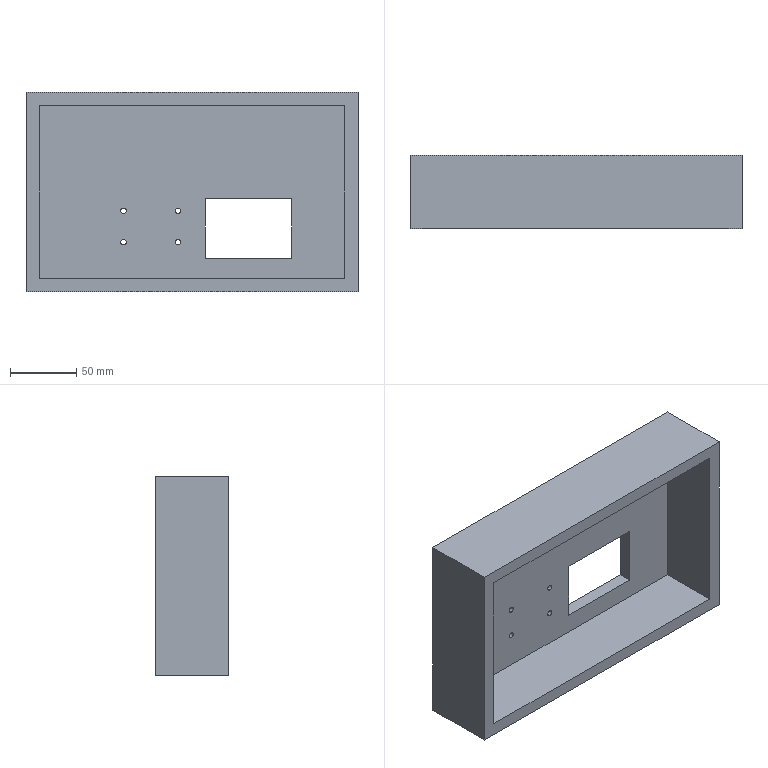Part | SolidWorks | features ICE 2, Cut 1, Extrusion 1 | 1 solid | 23 faces | box 250 x 55 x 150 mm | volume 687196 mm3 | plane 15 | cylinder 8 | commonest cylinder face diameters 4.2 x8
STEP:
#1=CARTESIAN_POINT('',(-42.988,58.447,39.302));
#2=VERTEX_POINT('',#1);
#3=CARTESIAN_POINT('',(-42.988,58.447,35.102));
#4=VERTEX_POINT('',#3);
#5=CARTESIAN_POINT('',(-42.988,58.447,37.202));
#6=DIRECTION('',(0.,-1.,0.));
#7=DIRECTION('',(0.,0.,1.));
#8=AXIS2_PLACEMENT_3D('',#5,#6,#7);
#9=CIRCLE('',#8,2.1);
#10=EDGE_CURVE('',#2,#4,#9,.T.);
#11=ORIENTED_EDGE('',*,*,#10,.T.);
#12=CARTESIAN_POINT('',(-42.988,68.447,35.102));
#13=VERTEX_POINT('',#12);
#14=CARTESIAN_POINT('',(-42.988,52.508,35.102));
#15=DIRECTION('',(0.,1.,0.));
#16=VECTOR('',#15,1000.);
#17=LINE('',#14,#16);
#18=EDGE_CURVE('',#4,#13,#17,.T.);
#19=ORIENTED_EDGE('',*,*,#18,.T.);
#20=CARTESIAN_POINT('',(-42.988,68.447,39.302));
#21=VERTEX_POINT('',#20);
#22=CARTESIAN_POINT('',(-42.988,68.447,37.202));
#23=DIRECTION('',(0.,-1.,0.));
#24=DIRECTION('',(0.,0.,-1.));
#25=AXIS2_PLACEMENT_3D('',#22,#23,#24);
#26=CIRCLE('',#25,2.1);
#27=EDGE_CURVE('',#21,#13,#26,.T.);
#28=ORIENTED_EDGE('',*,*,#27,.F.);
#29=CARTESIAN_POINT('',(-42.988,52.508,39.302));
#30=DIRECTION('',(0.,1.,0.));
#31=VECTOR('',#30,1000.);
#32=LINE('',#29,#31);
#33=EDGE_CURVE('',#2,#21,#32,.T.);
#34=ORIENTED_EDGE('',*,*,#33,.F.);
#35=EDGE_LOOP('',(#11,#19,#28,#34));
#36=FACE_OUTER_BOUND('',#35,.T.);
#37=CARTESIAN_POINT('',(-42.988,52.508,37.202));
#38=DIRECTION('',(0.,1.,0.));
#39=DIRECTION('',(0.,0.,1.));
#40=AXIS2_PLACEMENT_3D('',#37,#38,#39);
#41=CYLINDRICAL_SURFACE('',#40,2.1);
#42=ADVANCED_FACE('',(#36),#41,.F.);
#43=CARTESIAN_POINT('',(-42.988,58.447,62.952));
#44=VERTEX_POINT('',#43);
#45=CARTESIAN_POINT('',(-42.988,58.447,58.752));
#46=VERTEX_POINT('',#45);
#47=CARTESIAN_POINT('',(-42.988,58.447,60.852));
#48=DIRECTION('',(0.,-1.,0.));
#49=DIRECTION('',(0.,0.,1.));
#50=AXIS2_PLACEMENT_3D('',#47,#48,#49);
#51=CIRCLE('',#50,2.1);
#52=EDGE_CURVE('',#44,#46,#51,.T.);
#53=ORIENTED_EDGE('',*,*,#52,.T.);
#54=CARTESIAN_POINT('',(-42.988,68.447,58.752));
#55=VERTEX_POINT('',#54);
#56=CARTESIAN_POINT('',(-42.988,52.508,58.752));
#57=DIRECTION('',(0.,1.,0.));
#58=VECTOR('',#57,1000.);
#59=LINE('',#56,#58);
#60=EDGE_CURVE('',#46,#55,#59,.T.);
#61=ORIENTED_EDGE('',*,*,#60,.T.);
#62=CARTESIAN_POINT('',(-42.988,68.447,62.952));
#63=VERTEX_POINT('',#62);
#64=CARTESIAN_POINT('',(-42.988,68.447,60.852));
#65=DIRECTION('',(0.,-1.,0.));
#66=DIRECTION('',(0.,0.,-1.));
#67=AXIS2_PLACEMENT_3D('',#64,#65,#66);
#68=CIRCLE('',#67,2.1);
#69=EDGE_CURVE('',#63,#55,#68,.T.);
#70=ORIENTED_EDGE('',*,*,#69,.F.);
#71=CARTESIAN_POINT('',(-42.988,52.508,62.952));
#72=DIRECTION('',(0.,1.,0.));
#73=VECTOR('',#72,1000.);
#74=LINE('',#71,#73);
#75=EDGE_CURVE('',#44,#63,#74,.T.);
#76=ORIENTED_EDGE('',*,*,#75,.F.);
#77=EDGE_LOOP('',(#53,#61,#70,#76));
#78=FACE_OUTER_BOUND('',#77,.T.);
#79=CARTESIAN_POINT('',(-42.988,52.508,60.852));
#80=DIRECTION('',(0.,1.,0.));
#81=DIRECTION('',(0.,0.,1.));
#82=AXIS2_PLACEMENT_3D('',#79,#80,#81);
#83=CYLINDRICAL_SURFACE('',#82,2.1);
#84=ADVANCED_FACE('',(#78),#83,.F.);
#85=CARTESIAN_POINT('',(-83.988,58.447,62.952));
#86=VERTEX_POINT('',#85);
#87=CARTESIAN_POINT('',(-83.988,58.447,58.752));
#88=VERTEX_POINT('',#87);
#89=CARTESIAN_POINT('',(-83.988,58.447,60.852));
#90=DIRECTION('',(0.,-1.,0.));
#91=DIRECTION('',(0.,0.,1.));
#92=AXIS2_PLACEMENT_3D('',#89,#90,#91);
#93=CIRCLE('',#92,2.1);
#94=EDGE_CURVE('',#86,#88,#93,.T.);
#95=ORIENTED_EDGE('',*,*,#94,.T.);
#96=CARTESIAN_POINT('',(-83.988,68.447,58.752));
#97=VERTEX_POINT('',#96);
#98=CARTESIAN_POINT('',(-83.988,52.508,58.752));
#99=DIRECTION('',(0.,1.,0.));
#100=VECTOR('',#99,1000.);
#101=LINE('',#98,#100);
#102=EDGE_CURVE('',#88,#97,#101,.T.);
#103=ORIENTED_EDGE('',*,*,#102,.T.);
#104=CARTESIAN_POINT('',(-83.988,68.447,62.952));
#105=VERTEX_POINT('',#104);
#106=CARTESIAN_POINT('',(-83.988,68.447,60.852));
#107=DIRECTION('',(0.,-1.,0.));
#108=DIRECTION('',(0.,0.,-1.));
#109=AXIS2_PLACEMENT_3D('',#106,#107,#108);
#110=CIRCLE('',#109,2.1);
#111=EDGE_CURVE('',#105,#97,#110,.T.);
#112=ORIENTED_EDGE('',*,*,#111,.F.);
#113=CARTESIAN_POINT('',(-83.988,52.508,62.952));
#114=DIRECTION('',(0.,1.,0.));
#115=VECTOR('',#114,1000.);
#116=LINE('',#113,#115);
#117=EDGE_CURVE('',#86,#105,#116,.T.);
#118=ORIENTED_EDGE('',*,*,#117,.F.);
#119=EDGE_LOOP('',(#95,#103,#112,#118));
#120=FACE_OUTER_BOUND('',#119,.T.);
#121=CARTESIAN_POINT('',(-83.988,52.508,60.852));
#122=DIRECTION('',(0.,1.,0.));
#123=DIRECTION('',(0.,0.,1.));
#124=AXIS2_PLACEMENT_3D('',#121,#122,#123);
#125=CYLINDRICAL_SURFACE('',#124,2.1);
#126=ADVANCED_FACE('',(#120),#125,.F.);
#127=CARTESIAN_POINT('',(-83.988,58.447,39.302));
#128=VERTEX_POINT('',#127);
#129=CARTESIAN_POINT('',(-83.988,58.447,35.102));
#130=VERTEX_POINT('',#129);
#131=CARTESIAN_POINT('',(-83.988,58.447,37.202));
#132=DIRECTION('',(0.,-1.,0.));
#133=DIRECTION('',(0.,0.,1.));
#134=AXIS2_PLACEMENT_3D('',#131,#132,#133);
#135=CIRCLE('',#134,2.1);
#136=EDGE_CURVE('',#128,#130,#135,.T.);
#137=ORIENTED_EDGE('',*,*,#136,.T.);
#138=CARTESIAN_POINT('',(-83.988,68.447,35.102));
#139=VERTEX_POINT('',#138);
#140=CARTESIAN_POINT('',(-83.988,52.508,35.102));
#141=DIRECTION('',(0.,1.,0.));
#142=VECTOR('',#141,1000.);
#143=LINE('',#140,#142);
#144=EDGE_CURVE('',#130,#139,#143,.T.);
#145=ORIENTED_EDGE('',*,*,#144,.T.);
#146=CARTESIAN_POINT('',(-83.988,68.447,39.302));
#147=VERTEX_POINT('',#146);
#148=CARTESIAN_POINT('',(-83.988,68.447,37.202));
#149=DIRECTION('',(0.,-1.,0.));
#150=DIRECTION('',(0.,0.,-1.));
#151=AXIS2_PLACEMENT_3D('',#148,#149,#150);
#152=CIRCLE('',#151,2.1);
#153=EDGE_CURVE('',#147,#139,#152,.T.);
#154=ORIENTED_EDGE('',*,*,#153,.F.);
#155=CARTESIAN_POINT('',(-83.988,52.508,39.302));
#156=DIRECTION('',(0.,1.,0.));
#157=VECTOR('',#156,1000.);
#158=LINE('',#155,#157);
#159=EDGE_CURVE('',#128,#147,#158,.T.);
#160=ORIENTED_EDGE('',*,*,#159,.F.);
#161=EDGE_LOOP('',(#137,#145,#154,#160));
#162=FACE_OUTER_BOUND('',#161,.T.);
#163=CARTESIAN_POINT('',(-83.988,52.508,37.202));
#164=DIRECTION('',(0.,1.,0.));
#165=DIRECTION('',(0.,0.,1.));
#166=AXIS2_PLACEMENT_3D('',#163,#164,#165);
#167=CYLINDRICAL_SURFACE('',#166,2.1);
#168=ADVANCED_FACE('',(#162),#167,.F.);
#169=CARTESIAN_POINT('',(-157.482,68.447,0.));
#170=VERTEX_POINT('',#169);
#171=CARTESIAN_POINT('',(-157.482,13.447,0.));
#172=VERTEX_POINT('',#171);
#173=CARTESIAN_POINT('',(-157.482,68.447,0.));
#174=DIRECTION('',(0.,-1.,0.));
#175=VECTOR('',#174,1000.);
#176=LINE('',#173,#175);
#177=EDGE_CURVE('',#170,#172,#176,.T.);
#178=ORIENTED_EDGE('',*,*,#177,.T.);
#179=CARTESIAN_POINT('',(-157.482,13.447,150.));
#180=VERTEX_POINT('',#179);
#181=CARTESIAN_POINT('',(-157.482,13.447,150.));
#182=DIRECTION('',(0.,0.,-1.));
#183=VECTOR('',#182,1000.);
#184=LINE('',#181,#183);
#185=EDGE_CURVE('',#180,#172,#184,.T.);
#186=ORIENTED_EDGE('',*,*,#185,.F.);
#187=CARTESIAN_POINT('',(-157.482,68.447,150.));
#188=VERTEX_POINT('',#187);
#189=CARTESIAN_POINT('',(-157.482,68.447,150.));
#190=DIRECTION('',(0.,-1.,0.));
#191=VECTOR('',#190,1000.);
#192=LINE('',#189,#191);
#193=EDGE_CURVE('',#188,#180,#192,.T.);
#194=ORIENTED_EDGE('',*,*,#193,.F.);
#195=CARTESIAN_POINT('',(-157.482,68.447,150.));
#196=DIRECTION('',(0.,0.,-1.));
#197=VECTOR('',#196,1000.);
#198=LINE('',#195,#197);
#199=EDGE_CURVE('',#188,#170,#198,.T.);
#200=ORIENTED_EDGE('',*,*,#199,.T.);
#201=EDGE_LOOP('',(#178,#186,#194,#200));
#202=FACE_OUTER_BOUND('',#201,.T.);
#203=CARTESIAN_POINT('',(-157.482,68.447,150.));
#204=DIRECTION('',(1.,0.,0.));
#205=DIRECTION('',(0.,0.,-1.));
#206=AXIS2_PLACEMENT_3D('',#203,#204,#205);
#207=PLANE('',#206);
#208=ADVANCED_FACE('',(#202),#207,.F.);
#209=CARTESIAN_POINT('',(-147.482,13.447,10.));
#210=VERTEX_POINT('',#209);
#211=CARTESIAN_POINT('',(82.518,13.447,10.));
#212=VERTEX_POINT('',#211);
#213=CARTESIAN_POINT('',(82.518,13.447,10.));
#214=DIRECTION('',(1.,0.,0.));
#215=VECTOR('',#214,1000.);
#216=LINE('',#213,#215);
#217=EDGE_CURVE('',#210,#212,#216,.T.);
#218=ORIENTED_EDGE('',*,*,#217,.F.);
#219=CARTESIAN_POINT('',(-147.482,13.447,140.));
#220=VERTEX_POINT('',#219);
#221=CARTESIAN_POINT('',(-147.482,13.447,140.));
#222=DIRECTION('',(0.,0.,-1.));
#223=VECTOR('',#222,1000.);
#224=LINE('',#221,#223);
#225=EDGE_CURVE('',#220,#210,#224,.T.);
#226=ORIENTED_EDGE('',*,*,#225,.F.);
#227=CARTESIAN_POINT('',(82.518,13.447,140.));
#228=VERTEX_POINT('',#227);
#229=CARTESIAN_POINT('',(-147.482,13.447,140.));
#230=DIRECTION('',(-1.,0.,0.));
#231=VECTOR('',#230,1000.);
#232=LINE('',#229,#231);
#233=EDGE_CURVE('',#228,#220,#232,.T.);
#234=ORIENTED_EDGE('',*,*,#233,.F.);
#235=CARTESIAN_POINT('',(82.518,13.447,140.));
#236=DIRECTION('',(0.,0.,1.));
#237=VECTOR('',#236,1000.);
#238=LINE('',#235,#237);
#239=EDGE_CURVE('',#212,#228,#238,.T.);
#240=ORIENTED_EDGE('',*,*,#239,.F.);
#241=EDGE_LOOP('',(#218,#226,#234,#240));
#242=FACE_BOUND('',#241,.T.);
#243=CARTESIAN_POINT('',(92.518,13.447,0.));
#244=VERTEX_POINT('',#243);
#245=CARTESIAN_POINT('',(-157.482,13.447,0.));
#246=DIRECTION('',(1.,0.,0.));
#247=VECTOR('',#246,1000.);
#248=LINE('',#245,#247);
#249=EDGE_CURVE('',#172,#244,#248,.T.);
#250=ORIENTED_EDGE('',*,*,#249,.T.);
#251=CARTESIAN_POINT('',(92.518,13.447,150.));
#252=VERTEX_POINT('',#251);
#253=CARTESIAN_POINT('',(92.518,13.447,150.));
#254=DIRECTION('',(0.,0.,-1.));
#255=VECTOR('',#254,1000.);
#256=LINE('',#253,#255);
#257=EDGE_CURVE('',#252,#244,#256,.T.);
#258=ORIENTED_EDGE('',*,*,#257,.F.);
#259=CARTESIAN_POINT('',(-157.482,13.447,150.));
#260=DIRECTION('',(1.,0.,0.));
#261=VECTOR('',#260,1000.);
#262=LINE('',#259,#261);
#263=EDGE_CURVE('',#180,#252,#262,.T.);
#264=ORIENTED_EDGE('',*,*,#263,.F.);
#265=ORIENTED_EDGE('',*,*,#185,.T.);
#266=EDGE_LOOP('',(#250,#258,#264,#265));
#267=FACE_OUTER_BOUND('',#266,.T.);
#268=CARTESIAN_POINT('',(-157.482,13.447,150.));
#269=DIRECTION('',(0.,1.,0.));
#270=DIRECTION('',(0.,0.,1.));
#271=AXIS2_PLACEMENT_3D('',#268,#269,#270);
#272=PLANE('',#271);
#273=ADVANCED_FACE('',(#242,#267),#272,.F.);
#274=CARTESIAN_POINT('',(92.518,68.447,0.));
#275=VERTEX_POINT('',#274);
#276=CARTESIAN_POINT('',(92.518,68.447,0.));
#277=DIRECTION('',(0.,1.,0.));
#278=VECTOR('',#277,1000.);
#279=LINE('',#276,#278);
#280=EDGE_CURVE('',#244,#275,#279,.T.);
#281=ORIENTED_EDGE('',*,*,#280,.T.);
#282=CARTESIAN_POINT('',(92.518,68.447,150.));
#283=VERTEX_POINT('',#282);
#284=CARTESIAN_POINT('',(92.518,68.447,150.));
#285=DIRECTION('',(0.,0.,-1.));
#286=VECTOR('',#285,1000.);
#287=LINE('',#284,#286);
#288=EDGE_CURVE('',#283,#275,#287,.T.);
#289=ORIENTED_EDGE('',*,*,#288,.F.);
#290=CARTESIAN_POINT('',(92.518,68.447,150.));
#291=DIRECTION('',(0.,1.,0.));
#292=VECTOR('',#291,1000.);
#293=LINE('',#290,#292);
#294=EDGE_CURVE('',#252,#283,#293,.T.);
#295=ORIENTED_EDGE('',*,*,#294,.F.);
#296=ORIENTED_EDGE('',*,*,#257,.T.);
#297=EDGE_LOOP('',(#281,#289,#295,#296));
#298=FACE_OUTER_BOUND('',#297,.T.);
#299=CARTESIAN_POINT('',(92.518,68.447,150.));
#300=DIRECTION('',(-1.,0.,0.));
#301=DIRECTION('',(0.,-1.,0.));
#302=AXIS2_PLACEMENT_3D('',#299,#300,#301);
#303=PLANE('',#302);
#304=ADVANCED_FACE('',(#298),#303,.F.);
#305=ORIENTED_EDGE('',*,*,#27,.T.);
#306=CARTESIAN_POINT('',(-42.988,68.447,37.202));
#307=DIRECTION('',(0.,-1.,0.));
#308=DIRECTION('',(0.,0.,-1.));
#309=AXIS2_PLACEMENT_3D('',#306,#307,#308);
#310=CIRCLE('',#309,2.1);
#311=EDGE_CURVE('',#13,#21,#310,.T.);
#312=ORIENTED_EDGE('',*,*,#311,.T.);
#313=EDGE_LOOP('',(#305,#312));
#314=FACE_BOUND('',#313,.T.);
#315=ORIENTED_EDGE('',*,*,#69,.T.);
#316=CARTESIAN_POINT('',(-42.988,68.447,60.852));
#317=DIRECTION('',(0.,-1.,0.));
#318=DIRECTION('',(0.,0.,-1.));
#319=AXIS2_PLACEMENT_3D('',#316,#317,#318);
#320=CIRCLE('',#319,2.1);
#321=EDGE_CURVE('',#55,#63,#320,.T.);
#322=ORIENTED_EDGE('',*,*,#321,.T.);
#323=EDGE_LOOP('',(#315,#322));
#324=FACE_BOUND('',#323,.T.);
#325=ORIENTED_EDGE('',*,*,#111,.T.);
#326=CARTESIAN_POINT('',(-83.988,68.447,60.852));
#327=DIRECTION('',(0.,-1.,0.));
#328=DIRECTION('',(0.,0.,-1.));
#329=AXIS2_PLACEMENT_3D('',#326,#327,#328);
#330=CIRCLE('',#329,2.1);
#331=EDGE_CURVE('',#97,#105,#330,.T.);
#332=ORIENTED_EDGE('',*,*,#331,.T.);
#333=EDGE_LOOP('',(#325,#332));
#334=FACE_BOUND('',#333,.T.);
#335=ORIENTED_EDGE('',*,*,#153,.T.);
#336=CARTESIAN_POINT('',(-83.988,68.447,37.202));
#337=DIRECTION('',(0.,-1.,0.));
#338=DIRECTION('',(0.,0.,-1.));
#339=AXIS2_PLACEMENT_3D('',#336,#337,#338);
#340=CIRCLE('',#339,2.1);
#341=EDGE_CURVE('',#139,#147,#340,.T.);
#342=ORIENTED_EDGE('',*,*,#341,.T.);
#343=EDGE_LOOP('',(#335,#342));
#344=FACE_BOUND('',#343,.T.);
#345=CARTESIAN_POINT('',(42.518,68.447,70.));
#346=VERTEX_POINT('',#345);
#347=CARTESIAN_POINT('',(-22.482,68.447,70.));
#348=VERTEX_POINT('',#347);
#349=CARTESIAN_POINT('',(-22.482,68.447,70.));
#350=DIRECTION('',(-1.,0.,0.));
#351=VECTOR('',#350,1000.);
#352=LINE('',#349,#351);
#353=EDGE_CURVE('',#346,#348,#352,.T.);
#354=ORIENTED_EDGE('',*,*,#353,.T.);
#355=CARTESIAN_POINT('',(-22.482,68.447,25.));
#356=VERTEX_POINT('',#355);
#357=CARTESIAN_POINT('',(-22.482,68.447,70.));
#358=DIRECTION('',(0.,0.,-1.));
#359=VECTOR('',#358,1000.);
#360=LINE('',#357,#359);
#361=EDGE_CURVE('',#348,#356,#360,.T.);
#362=ORIENTED_EDGE('',*,*,#361,.T.);
#363=CARTESIAN_POINT('',(42.518,68.447,25.));
#364=VERTEX_POINT('',#363);
#365=CARTESIAN_POINT('',(-22.482,68.447,25.));
#366=DIRECTION('',(1.,0.,0.));
#367=VECTOR('',#366,1000.);
#368=LINE('',#365,#367);
#369=EDGE_CURVE('',#356,#364,#368,.T.);
#370=ORIENTED_EDGE('',*,*,#369,.T.);
#371=CARTESIAN_POINT('',(42.518,68.447,70.));
#372=DIRECTION('',(0.,0.,1.));
#373=VECTOR('',#372,1000.);
#374=LINE('',#371,#373);
#375=EDGE_CURVE('',#364,#346,#374,.T.);
#376=ORIENTED_EDGE('',*,*,#375,.T.);
#377=EDGE_LOOP('',(#354,#362,#370,#376));
#378=FACE_BOUND('',#377,.T.);
#379=CARTESIAN_POINT('',(-157.482,68.447,0.));
#380=DIRECTION('',(-1.,0.,0.));
#381=VECTOR('',#380,1000.);
#382=LINE('',#379,#381);
#383=EDGE_CURVE('',#275,#170,#382,.T.);
#384=ORIENTED_EDGE('',*,*,#383,.T.);
#385=ORIENTED_EDGE('',*,*,#199,.F.);
#386=CARTESIAN_POINT('',(-157.482,68.447,150.));
#387=DIRECTION('',(-1.,0.,0.));
#388=VECTOR('',#387,1000.);
#389=LINE('',#386,#388);
#390=EDGE_CURVE('',#283,#188,#389,.T.);
#391=ORIENTED_EDGE('',*,*,#390,.F.);
#392=ORIENTED_EDGE('',*,*,#288,.T.);
#393=EDGE_LOOP('',(#384,#385,#391,#392));
#394=FACE_OUTER_BOUND('',#393,.T.);
#395=CARTESIAN_POINT('',(-157.482,68.447,150.));
#396=DIRECTION('',(0.,-1.,0.));
#397=DIRECTION('',(0.,0.,-1.));
#398=AXIS2_PLACEMENT_3D('',#395,#396,#397);
#399=PLANE('',#398);
#400=ADVANCED_FACE('',(#314,#324,#334,#344,#378,#394),#399,.F.);
#401=ORIENTED_EDGE('',*,*,#193,.T.);
#402=ORIENTED_EDGE('',*,*,#263,.T.);
#403=ORIENTED_EDGE('',*,*,#294,.T.);
#404=ORIENTED_EDGE('',*,*,#390,.T.);
#405=EDGE_LOOP('',(#401,#402,#403,#404));
#406=FACE_OUTER_BOUND('',#405,.T.);
#407=CARTESIAN_POINT('',(0.,0.,150.));
#408=DIRECTION('',(0.,0.,1.));
#409=DIRECTION('',(1.,0.,0.));
#410=AXIS2_PLACEMENT_3D('',#407,#408,#409);
#411=PLANE('',#410);
#412=ADVANCED_FACE('',(#406),#411,.T.);
#413=ORIENTED_EDGE('',*,*,#177,.F.);
#414=ORIENTED_EDGE('',*,*,#383,.F.);
#415=ORIENTED_EDGE('',*,*,#280,.F.);
#416=ORIENTED_EDGE('',*,*,#249,.F.);
#417=EDGE_LOOP('',(#413,#414,#415,#416));
#418=FACE_OUTER_BOUND('',#417,.T.);
#419=CARTESIAN_POINT('',(0.,0.,0.));
#420=DIRECTION('',(0.,0.,1.));
#421=DIRECTION('',(1.,0.,0.));
#422=AXIS2_PLACEMENT_3D('',#419,#420,#421);
#423=PLANE('',#422);
#424=ADVANCED_FACE('',(#418),#423,.F.);
#425=ORIENTED_EDGE('',*,*,#225,.T.);
#426=CARTESIAN_POINT('',(-147.482,58.447,10.));
#427=VERTEX_POINT('',#426);
#428=CARTESIAN_POINT('',(-147.482,58.447,10.));
#429=DIRECTION('',(0.,-1.,0.));
#430=VECTOR('',#429,1000.);
#431=LINE('',#428,#430);
#432=EDGE_CURVE('',#427,#210,#431,.T.);
#433=ORIENTED_EDGE('',*,*,#432,.F.);
#434=CARTESIAN_POINT('',(-147.482,58.447,140.));
#435=VERTEX_POINT('',#434);
#436=CARTESIAN_POINT('',(-147.482,58.447,140.));
#437=DIRECTION('',(0.,0.,-1.));
#438=VECTOR('',#437,1000.);
#439=LINE('',#436,#438);
#440=EDGE_CURVE('',#435,#427,#439,.T.);
#441=ORIENTED_EDGE('',*,*,#440,.F.);
#442=CARTESIAN_POINT('',(-147.482,58.447,140.));
#443=DIRECTION('',(0.,-1.,0.));
#444=VECTOR('',#443,1000.);
#445=LINE('',#442,#444);
#446=EDGE_CURVE('',#435,#220,#445,.T.);
#447=ORIENTED_EDGE('',*,*,#446,.T.);
#448=EDGE_LOOP('',(#425,#433,#441,#447));
#449=FACE_OUTER_BOUND('',#448,.T.);
#450=CARTESIAN_POINT('',(-147.482,58.447,140.));
#451=DIRECTION('',(-1.,0.,0.));
#452=DIRECTION('',(0.,0.,1.));
#453=AXIS2_PLACEMENT_3D('',#450,#451,#452);
#454=PLANE('',#453);
#455=ADVANCED_FACE('',(#449),#454,.F.);
#456=ORIENTED_EDGE('',*,*,#233,.T.);
#457=ORIENTED_EDGE('',*,*,#446,.F.);
#458=CARTESIAN_POINT('',(82.518,58.447,140.));
#459=VERTEX_POINT('',#458);
#460=CARTESIAN_POINT('',(-147.482,58.447,140.));
#461=DIRECTION('',(-1.,0.,0.));
#462=VECTOR('',#461,1000.);
#463=LINE('',#460,#462);
#464=EDGE_CURVE('',#459,#435,#463,.T.);
#465=ORIENTED_EDGE('',*,*,#464,.F.);
#466=CARTESIAN_POINT('',(82.518,58.447,140.));
#467=DIRECTION('',(0.,-1.,0.));
#468=VECTOR('',#467,1000.);
#469=LINE('',#466,#468);
#470=EDGE_CURVE('',#459,#228,#469,.T.);
#471=ORIENTED_EDGE('',*,*,#470,.T.);
#472=EDGE_LOOP('',(#456,#457,#465,#471));
#473=FACE_OUTER_BOUND('',#472,.T.);
#474=CARTESIAN_POINT('',(-147.482,58.447,140.));
#475=DIRECTION('',(0.,0.,1.));
#476=DIRECTION('',(1.,0.,0.));
#477=AXIS2_PLACEMENT_3D('',#474,#475,#476);
#478=PLANE('',#477);
#479=ADVANCED_FACE('',(#473),#478,.F.);
#480=ORIENTED_EDGE('',*,*,#239,.T.);
#481=ORIENTED_EDGE('',*,*,#470,.F.);
#482=CARTESIAN_POINT('',(82.518,58.447,10.));
#483=VERTEX_POINT('',#482);
#484=CARTESIAN_POINT('',(82.518,58.447,140.));
#485=DIRECTION('',(0.,0.,1.));
#486=VECTOR('',#485,1000.);
#487=LINE('',#484,#486);
#488=EDGE_CURVE('',#483,#459,#487,.T.);
#489=ORIENTED_EDGE('',*,*,#488,.F.);
#490=CARTESIAN_POINT('',(82.518,58.447,10.));
#491=DIRECTION('',(0.,-1.,0.));
#492=VECTOR('',#491,1000.);
#493=LINE('',#490,#492);
#494=EDGE_CURVE('',#483,#212,#493,.T.);
#495=ORIENTED_EDGE('',*,*,#494,.T.);
#496=EDGE_LOOP('',(#480,#481,#489,#495));
#497=FACE_OUTER_BOUND('',#496,.T.);
#498=CARTESIAN_POINT('',(82.518,58.447,140.));
#499=DIRECTION('',(1.,0.,0.));
#500=DIRECTION('',(0.,0.,-1.));
#501=AXIS2_PLACEMENT_3D('',#498,#499,#500);
#502=PLANE('',#501);
#503=ADVANCED_FACE('',(#497),#502,.F.);
#504=ORIENTED_EDGE('',*,*,#217,.T.);
#505=ORIENTED_EDGE('',*,*,#494,.F.);
#506=CARTESIAN_POINT('',(82.518,58.447,10.));
#507=DIRECTION('',(1.,0.,0.));
#508=VECTOR('',#507,1000.);
#509=LINE('',#506,#508);
#510=EDGE_CURVE('',#427,#483,#509,.T.);
#511=ORIENTED_EDGE('',*,*,#510,.F.);
#512=ORIENTED_EDGE('',*,*,#432,.T.);
#513=EDGE_LOOP('',(#504,#505,#511,#512));
#514=FACE_OUTER_BOUND('',#513,.T.);
#515=CARTESIAN_POINT('',(82.518,58.447,10.));
#516=DIRECTION('',(0.,0.,-1.));
#517=DIRECTION('',(-1.,0.,0.));
#518=AXIS2_PLACEMENT_3D('',#515,#516,#517);
#519=PLANE('',#518);
#520=ADVANCED_FACE('',(#514),#519,.F.);
#521=ORIENTED_EDGE('',*,*,#10,.F.);
#522=CARTESIAN_POINT('',(-42.988,58.447,37.202));
#523=DIRECTION('',(0.,-1.,0.));
#524=DIRECTION('',(0.,0.,1.));
#525=AXIS2_PLACEMENT_3D('',#522,#523,#524);
#526=CIRCLE('',#525,2.1);
#527=EDGE_CURVE('',#4,#2,#526,.T.);
#528=ORIENTED_EDGE('',*,*,#527,.F.);
#529=EDGE_LOOP('',(#521,#528));
#530=FACE_BOUND('',#529,.T.);
#531=ORIENTED_EDGE('',*,*,#52,.F.);
#532=CARTESIAN_POINT('',(-42.988,58.447,60.852));
#533=DIRECTION('',(0.,-1.,0.));
#534=DIRECTION('',(0.,0.,1.));
#535=AXIS2_PLACEMENT_3D('',#532,#533,#534);
#536=CIRCLE('',#535,2.1);
#537=EDGE_CURVE('',#46,#44,#536,.T.);
#538=ORIENTED_EDGE('',*,*,#537,.F.);
#539=EDGE_LOOP('',(#531,#538));
#540=FACE_BOUND('',#539,.T.);
#541=ORIENTED_EDGE('',*,*,#94,.F.);
#542=CARTESIAN_POINT('',(-83.988,58.447,60.852));
#543=DIRECTION('',(0.,-1.,0.));
#544=DIRECTION('',(0.,0.,1.));
#545=AXIS2_PLACEMENT_3D('',#542,#543,#544);
#546=CIRCLE('',#545,2.1);
#547=EDGE_CURVE('',#88,#86,#546,.T.);
#548=ORIENTED_EDGE('',*,*,#547,.F.);
#549=EDGE_LOOP('',(#541,#548));
#550=FACE_BOUND('',#549,.T.);
#551=ORIENTED_EDGE('',*,*,#136,.F.);
#552=CARTESIAN_POINT('',(-83.988,58.447,37.202));
#553=DIRECTION('',(0.,-1.,0.));
#554=DIRECTION('',(0.,0.,1.));
#555=AXIS2_PLACEMENT_3D('',#552,#553,#554);
#556=CIRCLE('',#555,2.1);
#557=EDGE_CURVE('',#130,#128,#556,.T.);
#558=ORIENTED_EDGE('',*,*,#557,.F.);
#559=EDGE_LOOP('',(#551,#558));
#560=FACE_BOUND('',#559,.T.);
#561=CARTESIAN_POINT('',(-22.482,58.447,25.));
#562=VERTEX_POINT('',#561);
#563=CARTESIAN_POINT('',(42.518,58.447,25.));
#564=VERTEX_POINT('',#563);
#565=CARTESIAN_POINT('',(-22.482,58.447,25.));
#566=DIRECTION('',(1.,0.,0.));
#567=VECTOR('',#566,1000.);
#568=LINE('',#565,#567);
#569=EDGE_CURVE('',#562,#564,#568,.T.);
#570=ORIENTED_EDGE('',*,*,#569,.F.);
#571=CARTESIAN_POINT('',(-22.482,58.447,70.));
#572=VERTEX_POINT('',#571);
#573=CARTESIAN_POINT('',(-22.482,58.447,70.));
#574=DIRECTION('',(0.,0.,-1.));
#575=VECTOR('',#574,1000.);
#576=LINE('',#573,#575);
#577=EDGE_CURVE('',#572,#562,#576,.T.);
#578=ORIENTED_EDGE('',*,*,#577,.F.);
#579=CARTESIAN_POINT('',(42.518,58.447,70.));
#580=VERTEX_POINT('',#579);
#581=CARTESIAN_POINT('',(-22.482,58.447,70.));
#582=DIRECTION('',(-1.,0.,0.));
#583=VECTOR('',#582,1000.);
#584=LINE('',#581,#583);
#585=EDGE_CURVE('',#580,#572,#584,.T.);
#586=ORIENTED_EDGE('',*,*,#585,.F.);
#587=CARTESIAN_POINT('',(42.518,58.447,70.));
#588=DIRECTION('',(0.,0.,1.));
#589=VECTOR('',#588,1000.);
#590=LINE('',#587,#589);
#591=EDGE_CURVE('',#564,#580,#590,.T.);
#592=ORIENTED_EDGE('',*,*,#591,.F.);
#593=EDGE_LOOP('',(#570,#578,#586,#592));
#594=FACE_BOUND('',#593,.T.);
#595=ORIENTED_EDGE('',*,*,#440,.T.);
#596=ORIENTED_EDGE('',*,*,#510,.T.);
#597=ORIENTED_EDGE('',*,*,#488,.T.);
#598=ORIENTED_EDGE('',*,*,#464,.T.);
#599=EDGE_LOOP('',(#595,#596,#597,#598));
#600=FACE_OUTER_BOUND('',#599,.T.);
#601=CARTESIAN_POINT('',(0.,58.447,0.));
#602=DIRECTION('',(0.,1.,0.));
#603=DIRECTION('',(0.,0.,1.));
#604=AXIS2_PLACEMENT_3D('',#601,#602,#603);
#605=PLANE('',#604);
#606=ADVANCED_FACE('',(#530,#540,#550,#560,#594,#600),#605,.F.);
#607=ORIENTED_EDGE('',*,*,#577,.T.);
#608=CARTESIAN_POINT('',(-22.482,68.447,25.));
#609=DIRECTION('',(0.,-1.,0.));
#610=VECTOR('',#609,1000.);
#611=LINE('',#608,#610);
#612=EDGE_CURVE('',#356,#562,#611,.T.);
#613=ORIENTED_EDGE('',*,*,#612,.F.);
#614=ORIENTED_EDGE('',*,*,#361,.F.);
#615=CARTESIAN_POINT('',(-22.482,68.447,70.));
#616=DIRECTION('',(0.,-1.,0.));
#617=VECTOR('',#616,1000.);
#618=LINE('',#615,#617);
#619=EDGE_CURVE('',#348,#572,#618,.T.);
#620=ORIENTED_EDGE('',*,*,#619,.T.);
#621=EDGE_LOOP('',(#607,#613,#614,#620));
#622=FACE_OUTER_BOUND('',#621,.T.);
#623=CARTESIAN_POINT('',(-22.482,68.447,70.));
#624=DIRECTION('',(-1.,0.,0.));
#625=DIRECTION('',(0.,0.,1.));
#626=AXIS2_PLACEMENT_3D('',#623,#624,#625);
#627=PLANE('',#626);
#628=ADVANCED_FACE('',(#622),#627,.F.);
#629=ORIENTED_EDGE('',*,*,#585,.T.);
#630=ORIENTED_EDGE('',*,*,#619,.F.);
#631=ORIENTED_EDGE('',*,*,#353,.F.);
#632=CARTESIAN_POINT('',(42.518,68.447,70.));
#633=DIRECTION('',(0.,-1.,0.));
#634=VECTOR('',#633,1000.);
#635=LINE('',#632,#634);
#636=EDGE_CURVE('',#346,#580,#635,.T.);
#637=ORIENTED_EDGE('',*,*,#636,.T.);
#638=EDGE_LOOP('',(#629,#630,#631,#637));
#639=FACE_OUTER_BOUND('',#638,.T.);
#640=CARTESIAN_POINT('',(-22.482,68.447,70.));
#641=DIRECTION('',(0.,0.,1.));
#642=DIRECTION('',(1.,0.,0.));
#643=AXIS2_PLACEMENT_3D('',#640,#641,#642);
#644=PLANE('',#643);
#645=ADVANCED_FACE('',(#639),#644,.F.);
#646=ORIENTED_EDGE('',*,*,#591,.T.);
#647=ORIENTED_EDGE('',*,*,#636,.F.);
#648=ORIENTED_EDGE('',*,*,#375,.F.);
#649=CARTESIAN_POINT('',(42.518,68.447,25.));
#650=DIRECTION('',(0.,-1.,0.));
#651=VECTOR('',#650,1000.);
#652=LINE('',#649,#651);
#653=EDGE_CURVE('',#364,#564,#652,.T.);
#654=ORIENTED_EDGE('',*,*,#653,.T.);
#655=EDGE_LOOP('',(#646,#647,#648,#654));
#656=FACE_OUTER_BOUND('',#655,.T.);
#657=CARTESIAN_POINT('',(42.518,68.447,70.));
#658=DIRECTION('',(1.,0.,0.));
#659=DIRECTION('',(0.,0.,-1.));
#660=AXIS2_PLACEMENT_3D('',#657,#658,#659);
#661=PLANE('',#660);
#662=ADVANCED_FACE('',(#656),#661,.F.);
#663=ORIENTED_EDGE('',*,*,#569,.T.);
#664=ORIENTED_EDGE('',*,*,#653,.F.);
#665=ORIENTED_EDGE('',*,*,#369,.F.);
#666=ORIENTED_EDGE('',*,*,#612,.T.);
#667=EDGE_LOOP('',(#663,#664,#665,#666));
#668=FACE_OUTER_BOUND('',#667,.T.);
#669=CARTESIAN_POINT('',(-22.482,68.447,25.));
#670=DIRECTION('',(0.,0.,-1.));
#671=DIRECTION('',(-1.,0.,0.));
#672=AXIS2_PLACEMENT_3D('',#669,#670,#671);
#673=PLANE('',#672);
#674=ADVANCED_FACE('',(#668),#673,.F.);
#675=ORIENTED_EDGE('',*,*,#144,.F.);
#676=ORIENTED_EDGE('',*,*,#557,.T.);
#677=ORIENTED_EDGE('',*,*,#159,.T.);
#678=ORIENTED_EDGE('',*,*,#341,.F.);
#679=EDGE_LOOP('',(#675,#676,#677,#678));
#680=FACE_OUTER_BOUND('',#679,.T.);
#681=CARTESIAN_POINT('',(-83.988,52.508,37.202));
#682=DIRECTION('',(0.,1.,0.));
#683=DIRECTION('',(0.,0.,1.));
#684=AXIS2_PLACEMENT_3D('',#681,#682,#683);
#685=CYLINDRICAL_SURFACE('',#684,2.1);
#686=ADVANCED_FACE('',(#680),#685,.F.);
#687=ORIENTED_EDGE('',*,*,#102,.F.);
#688=ORIENTED_EDGE('',*,*,#547,.T.);
#689=ORIENTED_EDGE('',*,*,#117,.T.);
#690=ORIENTED_EDGE('',*,*,#331,.F.);
#691=EDGE_LOOP('',(#687,#688,#689,#690));
#692=FACE_OUTER_BOUND('',#691,.T.);
#693=CARTESIAN_POINT('',(-83.988,52.508,60.852));
#694=DIRECTION('',(0.,1.,0.));
#695=DIRECTION('',(0.,0.,1.));
#696=AXIS2_PLACEMENT_3D('',#693,#694,#695);
#697=CYLINDRICAL_SURFACE('',#696,2.1);
#698=ADVANCED_FACE('',(#692),#697,.F.);
#699=ORIENTED_EDGE('',*,*,#60,.F.);
#700=ORIENTED_EDGE('',*,*,#537,.T.);
#701=ORIENTED_EDGE('',*,*,#75,.T.);
#702=ORIENTED_EDGE('',*,*,#321,.F.);
#703=EDGE_LOOP('',(#699,#700,#701,#702));
#704=FACE_OUTER_BOUND('',#703,.T.);
#705=CARTESIAN_POINT('',(-42.988,52.508,60.852));
#706=DIRECTION('',(0.,1.,0.));
#707=DIRECTION('',(0.,0.,1.));
#708=AXIS2_PLACEMENT_3D('',#705,#706,#707);
#709=CYLINDRICAL_SURFACE('',#708,2.1);
#710=ADVANCED_FACE('',(#704),#709,.F.);
#711=ORIENTED_EDGE('',*,*,#18,.F.);
#712=ORIENTED_EDGE('',*,*,#527,.T.);
#713=ORIENTED_EDGE('',*,*,#33,.T.);
#714=ORIENTED_EDGE('',*,*,#311,.F.);
#715=EDGE_LOOP('',(#711,#712,#713,#714));
#716=FACE_OUTER_BOUND('',#715,.T.);
#717=CARTESIAN_POINT('',(-42.988,52.508,37.202));
#718=DIRECTION('',(0.,1.,0.));
#719=DIRECTION('',(0.,0.,1.));
#720=AXIS2_PLACEMENT_3D('',#717,#718,#719);
#721=CYLINDRICAL_SURFACE('',#720,2.1);
#722=ADVANCED_FACE('',(#716),#721,.F.);
#723=CLOSED_SHELL('',(#42,#84,#126,#168,#208,#273,#304,#400,#412,#424,#455,#479,#503,#520,#606,#628,#645,#662,#674,#686,#698,#710,#722));
#724=MANIFOLD_SOLID_BREP('',#723);
#725=CARTESIAN_POINT('',(0.,0.,0.));
#726=DIRECTION('',(0.,0.,1.));
#727=DIRECTION('',(1.,0.,0.));
#728=AXIS2_PLACEMENT_3D('',#725,#726,#727);
#729=(LENGTH_UNIT()NAMED_UNIT(*)SI_UNIT(.MILLI.,.METRE.));
#730=UNCERTAINTY_MEASURE_WITH_UNIT(LENGTH_MEASURE(0.00001),#729,'','');
#731=(NAMED_UNIT(*)PLANE_ANGLE_UNIT()SI_UNIT($,.RADIAN.));
#732=(NAMED_UNIT(*)SI_UNIT($,.STERADIAN.)SOLID_ANGLE_UNIT());
#733=(GEOMETRIC_REPRESENTATION_CONTEXT(3)GLOBAL_UNCERTAINTY_ASSIGNED_CONTEXT((#730))GLOBAL_UNIT_ASSIGNED_CONTEXT((#729,#731,#732))REPRESENTATION_CONTEXT('',''));
#734=ADVANCED_BREP_SHAPE_REPRESENTATION('',(#724,#728),#733);